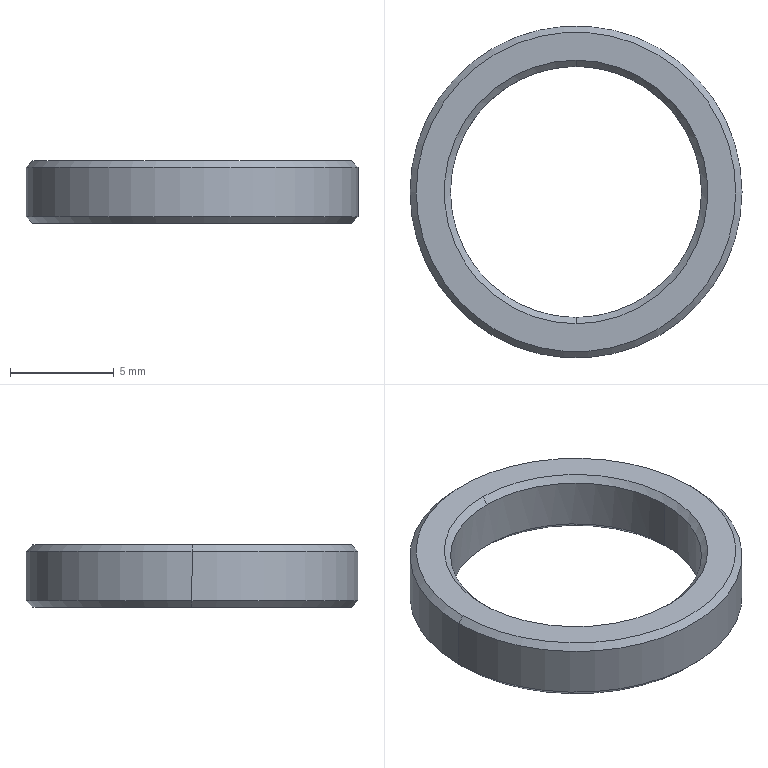Part | SolidWorks | features BaseBody 1 | 1 solid | 14 faces | box 16 x 16 x 3 mm | volume 250.27 mm3 | cone 8 | cylinder 4 | plane 2 | commonest cylinder face diameters 12.1 x2 16 x2
STEP:
#1=CARTESIAN_POINT('',(-8.,0.,2.7));
#2=VERTEX_POINT('',#1);
#3=CARTESIAN_POINT('',(8.,0.,2.7));
#4=VERTEX_POINT('',#3);
#5=CARTESIAN_POINT('',(0.,0.,2.7));
#6=DIRECTION('',(0.,0.,-1.));
#7=DIRECTION('',(-1.,0.,0.));
#8=AXIS2_PLACEMENT_3D('',#5,#6,#7);
#9=CIRCLE('',#8,8.);
#10=EDGE_CURVE('',#2,#4,#9,.T.);
#11=ORIENTED_EDGE('',*,*,#10,.T.);
#12=CARTESIAN_POINT('',(8.,0.,0.3));
#13=VERTEX_POINT('',#12);
#14=CARTESIAN_POINT('',(8.,0.,3.));
#15=DIRECTION('',(0.,0.,-1.));
#16=VECTOR('',#15,1000.);
#17=LINE('',#14,#16);
#18=EDGE_CURVE('',#4,#13,#17,.T.);
#19=ORIENTED_EDGE('',*,*,#18,.T.);
#20=CARTESIAN_POINT('',(-8.,0.,0.3));
#21=VERTEX_POINT('',#20);
#22=CARTESIAN_POINT('',(0.,0.,0.3));
#23=DIRECTION('',(0.,0.,1.));
#24=DIRECTION('',(-1.,0.,0.));
#25=AXIS2_PLACEMENT_3D('',#22,#23,#24);
#26=CIRCLE('',#25,8.);
#27=EDGE_CURVE('',#13,#21,#26,.T.);
#28=ORIENTED_EDGE('',*,*,#27,.T.);
#29=CARTESIAN_POINT('',(-8.,0.,3.));
#30=DIRECTION('',(0.,0.,-1.));
#31=VECTOR('',#30,1000.);
#32=LINE('',#29,#31);
#33=EDGE_CURVE('',#2,#21,#32,.T.);
#34=ORIENTED_EDGE('',*,*,#33,.F.);
#35=EDGE_LOOP('',(#11,#19,#28,#34));
#36=FACE_OUTER_BOUND('',#35,.T.);
#37=CARTESIAN_POINT('',(0.,0.,3.));
#38=DIRECTION('',(0.,0.,-1.));
#39=DIRECTION('',(-1.,0.,0.));
#40=AXIS2_PLACEMENT_3D('',#37,#38,#39);
#41=CYLINDRICAL_SURFACE('',#40,8.);
#42=ADVANCED_FACE('',(#36),#41,.T.);
#43=CARTESIAN_POINT('',(7.7,0.,0.));
#44=VERTEX_POINT('',#43);
#45=CARTESIAN_POINT('',(-7.7,0.,0.));
#46=VERTEX_POINT('',#45);
#47=CARTESIAN_POINT('',(0.,0.,0.));
#48=DIRECTION('',(0.,0.,1.));
#49=DIRECTION('',(1.,0.,0.));
#50=AXIS2_PLACEMENT_3D('',#47,#48,#49);
#51=CIRCLE('',#50,7.7);
#52=EDGE_CURVE('',#44,#46,#51,.T.);
#53=ORIENTED_EDGE('',*,*,#52,.T.);
#54=CARTESIAN_POINT('',(-8.,0.,0.3));
#55=DIRECTION('',(-0.7071,0.,0.7071));
#56=VECTOR('',#55,1000.);
#57=LINE('',#54,#56);
#58=EDGE_CURVE('',#46,#21,#57,.T.);
#59=ORIENTED_EDGE('',*,*,#58,.T.);
#60=ORIENTED_EDGE('',*,*,#27,.F.);
#61=CARTESIAN_POINT('',(8.,0.,0.3));
#62=DIRECTION('',(0.7071,0.,0.7071));
#63=VECTOR('',#62,1000.);
#64=LINE('',#61,#63);
#65=EDGE_CURVE('',#44,#13,#64,.T.);
#66=ORIENTED_EDGE('',*,*,#65,.F.);
#67=EDGE_LOOP('',(#53,#59,#60,#66));
#68=FACE_OUTER_BOUND('',#67,.T.);
#69=CARTESIAN_POINT('',(0.,0.,0.3));
#70=DIRECTION('',(0.,0.,1.));
#71=DIRECTION('',(1.,0.,0.));
#72=AXIS2_PLACEMENT_3D('',#69,#70,#71);
#73=CONICAL_SURFACE('',#72,8.,0.7854);
#74=ADVANCED_FACE('',(#68),#73,.T.);
#75=CARTESIAN_POINT('',(-7.7,0.,3.));
#76=VERTEX_POINT('',#75);
#77=CARTESIAN_POINT('',(7.7,0.,3.));
#78=VERTEX_POINT('',#77);
#79=CARTESIAN_POINT('',(0.,0.,3.));
#80=DIRECTION('',(0.,0.,-1.));
#81=DIRECTION('',(-1.,0.,0.));
#82=AXIS2_PLACEMENT_3D('',#79,#80,#81);
#83=CIRCLE('',#82,7.7);
#84=EDGE_CURVE('',#76,#78,#83,.T.);
#85=ORIENTED_EDGE('',*,*,#84,.T.);
#86=CARTESIAN_POINT('',(8.,0.,2.7));
#87=DIRECTION('',(0.7071,0.,-0.7071));
#88=VECTOR('',#87,1000.);
#89=LINE('',#86,#88);
#90=EDGE_CURVE('',#78,#4,#89,.T.);
#91=ORIENTED_EDGE('',*,*,#90,.T.);
#92=ORIENTED_EDGE('',*,*,#10,.F.);
#93=CARTESIAN_POINT('',(-8.,0.,2.7));
#94=DIRECTION('',(-0.7071,0.,-0.7071));
#95=VECTOR('',#94,1000.);
#96=LINE('',#93,#95);
#97=EDGE_CURVE('',#76,#2,#96,.T.);
#98=ORIENTED_EDGE('',*,*,#97,.F.);
#99=EDGE_LOOP('',(#85,#91,#92,#98));
#100=FACE_OUTER_BOUND('',#99,.T.);
#101=CARTESIAN_POINT('',(0.,0.,2.7));
#102=DIRECTION('',(0.,0.,-1.));
#103=DIRECTION('',(-1.,0.,0.));
#104=AXIS2_PLACEMENT_3D('',#101,#102,#103);
#105=CONICAL_SURFACE('',#104,8.,0.7854);
#106=ADVANCED_FACE('',(#100),#105,.T.);
#107=CARTESIAN_POINT('',(6.05,0.,0.3));
#108=VERTEX_POINT('',#107);
#109=CARTESIAN_POINT('',(-6.05,0.,0.3));
#110=VERTEX_POINT('',#109);
#111=CARTESIAN_POINT('',(0.,0.,0.3));
#112=DIRECTION('',(0.,0.,-1.));
#113=DIRECTION('',(-1.,0.,0.));
#114=AXIS2_PLACEMENT_3D('',#111,#112,#113);
#115=CIRCLE('',#114,6.05);
#116=EDGE_CURVE('',#108,#110,#115,.T.);
#117=ORIENTED_EDGE('',*,*,#116,.F.);
#118=CARTESIAN_POINT('',(6.35,0.,0.));
#119=VERTEX_POINT('',#118);
#120=CARTESIAN_POINT('',(6.35,0.,0.));
#121=DIRECTION('',(0.7071,0.,-0.7071));
#122=VECTOR('',#121,1000.);
#123=LINE('',#120,#122);
#124=EDGE_CURVE('',#108,#119,#123,.T.);
#125=ORIENTED_EDGE('',*,*,#124,.T.);
#126=CARTESIAN_POINT('',(-6.35,0.,0.));
#127=VERTEX_POINT('',#126);
#128=CARTESIAN_POINT('',(0.,0.,0.));
#129=DIRECTION('',(0.,0.,-1.));
#130=DIRECTION('',(-1.,0.,0.));
#131=AXIS2_PLACEMENT_3D('',#128,#129,#130);
#132=CIRCLE('',#131,6.35);
#133=EDGE_CURVE('',#119,#127,#132,.T.);
#134=ORIENTED_EDGE('',*,*,#133,.T.);
#135=CARTESIAN_POINT('',(-6.35,0.,0.));
#136=DIRECTION('',(-0.7071,0.,-0.7071));
#137=VECTOR('',#136,1000.);
#138=LINE('',#135,#137);
#139=EDGE_CURVE('',#110,#127,#138,.T.);
#140=ORIENTED_EDGE('',*,*,#139,.F.);
#141=EDGE_LOOP('',(#117,#125,#134,#140));
#142=FACE_OUTER_BOUND('',#141,.T.);
#143=CARTESIAN_POINT('',(0.,0.,0.));
#144=DIRECTION('',(0.,0.,-1.));
#145=DIRECTION('',(-1.,0.,0.));
#146=AXIS2_PLACEMENT_3D('',#143,#144,#145);
#147=CONICAL_SURFACE('',#146,6.35,0.7854);
#148=ADVANCED_FACE('',(#142),#147,.F.);
#149=CARTESIAN_POINT('',(0.,6.05,2.7));
#150=VERTEX_POINT('',#149);
#151=CARTESIAN_POINT('',(-6.05,0.,2.7));
#152=VERTEX_POINT('',#151);
#153=CARTESIAN_POINT('',(0.,0.,2.7));
#154=DIRECTION('',(0.,0.,1.));
#155=DIRECTION('',(1.,0.,0.));
#156=AXIS2_PLACEMENT_3D('',#153,#154,#155);
#157=CIRCLE('',#156,6.05);
#158=EDGE_CURVE('',#150,#152,#157,.T.);
#159=ORIENTED_EDGE('',*,*,#158,.F.);
#160=CARTESIAN_POINT('',(0.,6.35,3.));
#161=VERTEX_POINT('',#160);
#162=CARTESIAN_POINT('',(0.,6.35,3.));
#163=DIRECTION('',(0.,0.7071,0.7071));
#164=VECTOR('',#163,1000.);
#165=LINE('',#162,#164);
#166=EDGE_CURVE('',#150,#161,#165,.T.);
#167=ORIENTED_EDGE('',*,*,#166,.T.);
#168=CARTESIAN_POINT('',(0.,-6.35,3.));
#169=VERTEX_POINT('',#168);
#170=CARTESIAN_POINT('',(0.,0.,3.));
#171=DIRECTION('',(0.,0.,-1.));
#172=DIRECTION('',(0.,-1.,0.));
#173=AXIS2_PLACEMENT_3D('',#170,#171,#172);
#174=CIRCLE('',#173,6.35);
#175=EDGE_CURVE('',#169,#161,#174,.T.);
#176=ORIENTED_EDGE('',*,*,#175,.F.);
#177=CARTESIAN_POINT('',(0.,-6.05,2.7));
#178=VERTEX_POINT('',#177);
#179=CARTESIAN_POINT('',(0.,-6.35,3.));
#180=DIRECTION('',(0.,-0.7071,0.7071));
#181=VECTOR('',#180,1000.);
#182=LINE('',#179,#181);
#183=EDGE_CURVE('',#178,#169,#182,.T.);
#184=ORIENTED_EDGE('',*,*,#183,.F.);
#185=CARTESIAN_POINT('',(0.,0.,2.7));
#186=DIRECTION('',(0.,0.,1.));
#187=DIRECTION('',(1.,0.,0.));
#188=AXIS2_PLACEMENT_3D('',#185,#186,#187);
#189=CIRCLE('',#188,6.05);
#190=EDGE_CURVE('',#152,#178,#189,.T.);
#191=ORIENTED_EDGE('',*,*,#190,.F.);
#192=EDGE_LOOP('',(#159,#167,#176,#184,#191));
#193=FACE_OUTER_BOUND('',#192,.T.);
#194=CARTESIAN_POINT('',(0.,0.,3.));
#195=DIRECTION('',(0.,0.,1.));
#196=DIRECTION('',(0.,-1.,0.));
#197=AXIS2_PLACEMENT_3D('',#194,#195,#196);
#198=CONICAL_SURFACE('',#197,6.35,0.7854);
#199=ADVANCED_FACE('',(#193),#198,.F.);
#200=ORIENTED_EDGE('',*,*,#190,.T.);
#201=CARTESIAN_POINT('',(6.05,0.,2.7));
#202=VERTEX_POINT('',#201);
#203=CARTESIAN_POINT('',(0.,0.,2.7));
#204=DIRECTION('',(0.,0.,1.));
#205=DIRECTION('',(1.,0.,0.));
#206=AXIS2_PLACEMENT_3D('',#203,#204,#205);
#207=CIRCLE('',#206,6.05);
#208=EDGE_CURVE('',#178,#202,#207,.T.);
#209=ORIENTED_EDGE('',*,*,#208,.T.);
#210=CARTESIAN_POINT('',(6.05,0.,3.));
#211=DIRECTION('',(0.,0.,-1.));
#212=VECTOR('',#211,1000.);
#213=LINE('',#210,#212);
#214=EDGE_CURVE('',#202,#108,#213,.T.);
#215=ORIENTED_EDGE('',*,*,#214,.T.);
#216=ORIENTED_EDGE('',*,*,#116,.T.);
#217=CARTESIAN_POINT('',(-6.05,0.,3.));
#218=DIRECTION('',(0.,0.,-1.));
#219=VECTOR('',#218,1000.);
#220=LINE('',#217,#219);
#221=EDGE_CURVE('',#152,#110,#220,.T.);
#222=ORIENTED_EDGE('',*,*,#221,.F.);
#223=EDGE_LOOP('',(#200,#209,#215,#216,#222));
#224=FACE_OUTER_BOUND('',#223,.T.);
#225=CARTESIAN_POINT('',(0.,0.,3.));
#226=DIRECTION('',(0.,0.,-1.));
#227=DIRECTION('',(-1.,0.,0.));
#228=AXIS2_PLACEMENT_3D('',#225,#226,#227);
#229=CYLINDRICAL_SURFACE('',#228,6.05);
#230=ADVANCED_FACE('',(#224),#229,.F.);
#231=ORIENTED_EDGE('',*,*,#18,.F.);
#232=CARTESIAN_POINT('',(0.,0.,2.7));
#233=DIRECTION('',(0.,0.,-1.));
#234=DIRECTION('',(-1.,0.,0.));
#235=AXIS2_PLACEMENT_3D('',#232,#233,#234);
#236=CIRCLE('',#235,8.);
#237=EDGE_CURVE('',#4,#2,#236,.T.);
#238=ORIENTED_EDGE('',*,*,#237,.T.);
#239=ORIENTED_EDGE('',*,*,#33,.T.);
#240=CARTESIAN_POINT('',(0.,0.,0.3));
#241=DIRECTION('',(0.,0.,1.));
#242=DIRECTION('',(-1.,0.,0.));
#243=AXIS2_PLACEMENT_3D('',#240,#241,#242);
#244=CIRCLE('',#243,8.);
#245=EDGE_CURVE('',#21,#13,#244,.T.);
#246=ORIENTED_EDGE('',*,*,#245,.T.);
#247=EDGE_LOOP('',(#231,#238,#239,#246));
#248=FACE_OUTER_BOUND('',#247,.T.);
#249=CARTESIAN_POINT('',(0.,0.,3.));
#250=DIRECTION('',(0.,0.,-1.));
#251=DIRECTION('',(-1.,0.,0.));
#252=AXIS2_PLACEMENT_3D('',#249,#250,#251);
#253=CYLINDRICAL_SURFACE('',#252,8.);
#254=ADVANCED_FACE('',(#248),#253,.T.);
#255=ORIENTED_EDGE('',*,*,#58,.F.);
#256=CARTESIAN_POINT('',(0.,0.,0.));
#257=DIRECTION('',(0.,0.,1.));
#258=DIRECTION('',(1.,0.,0.));
#259=AXIS2_PLACEMENT_3D('',#256,#257,#258);
#260=CIRCLE('',#259,7.7);
#261=EDGE_CURVE('',#46,#44,#260,.T.);
#262=ORIENTED_EDGE('',*,*,#261,.T.);
#263=ORIENTED_EDGE('',*,*,#65,.T.);
#264=ORIENTED_EDGE('',*,*,#245,.F.);
#265=EDGE_LOOP('',(#255,#262,#263,#264));
#266=FACE_OUTER_BOUND('',#265,.T.);
#267=CARTESIAN_POINT('',(0.,0.,0.3));
#268=DIRECTION('',(0.,0.,1.));
#269=DIRECTION('',(1.,0.,0.));
#270=AXIS2_PLACEMENT_3D('',#267,#268,#269);
#271=CONICAL_SURFACE('',#270,8.,0.7854);
#272=ADVANCED_FACE('',(#266),#271,.T.);
#273=ORIENTED_EDGE('',*,*,#90,.F.);
#274=CARTESIAN_POINT('',(0.,0.,3.));
#275=DIRECTION('',(0.,0.,-1.));
#276=DIRECTION('',(-1.,0.,0.));
#277=AXIS2_PLACEMENT_3D('',#274,#275,#276);
#278=CIRCLE('',#277,7.7);
#279=EDGE_CURVE('',#78,#76,#278,.T.);
#280=ORIENTED_EDGE('',*,*,#279,.T.);
#281=ORIENTED_EDGE('',*,*,#97,.T.);
#282=ORIENTED_EDGE('',*,*,#237,.F.);
#283=EDGE_LOOP('',(#273,#280,#281,#282));
#284=FACE_OUTER_BOUND('',#283,.T.);
#285=CARTESIAN_POINT('',(0.,0.,2.7));
#286=DIRECTION('',(0.,0.,-1.));
#287=DIRECTION('',(-1.,0.,0.));
#288=AXIS2_PLACEMENT_3D('',#285,#286,#287);
#289=CONICAL_SURFACE('',#288,8.,0.7854);
#290=ADVANCED_FACE('',(#284),#289,.T.);
#291=CARTESIAN_POINT('',(0.,0.,0.));
#292=DIRECTION('',(0.,0.,-1.));
#293=DIRECTION('',(-1.,0.,0.));
#294=AXIS2_PLACEMENT_3D('',#291,#292,#293);
#295=CIRCLE('',#294,6.35);
#296=EDGE_CURVE('',#127,#119,#295,.T.);
#297=ORIENTED_EDGE('',*,*,#296,.F.);
#298=ORIENTED_EDGE('',*,*,#133,.F.);
#299=EDGE_LOOP('',(#297,#298));
#300=FACE_BOUND('',#299,.T.);
#301=ORIENTED_EDGE('',*,*,#52,.F.);
#302=ORIENTED_EDGE('',*,*,#261,.F.);
#303=EDGE_LOOP('',(#301,#302));
#304=FACE_OUTER_BOUND('',#303,.T.);
#305=CARTESIAN_POINT('',(0.,0.,0.));
#306=DIRECTION('',(0.,0.,1.));
#307=DIRECTION('',(1.,0.,0.));
#308=AXIS2_PLACEMENT_3D('',#305,#306,#307);
#309=PLANE('',#308);
#310=ADVANCED_FACE('',(#300,#304),#309,.F.);
#311=ORIENTED_EDGE('',*,*,#84,.F.);
#312=ORIENTED_EDGE('',*,*,#279,.F.);
#313=EDGE_LOOP('',(#311,#312));
#314=FACE_OUTER_BOUND('',#313,.T.);
#315=ORIENTED_EDGE('',*,*,#175,.T.);
#316=CARTESIAN_POINT('',(0.,0.,3.));
#317=DIRECTION('',(0.,0.,-1.));
#318=DIRECTION('',(0.,-1.,0.));
#319=AXIS2_PLACEMENT_3D('',#316,#317,#318);
#320=CIRCLE('',#319,6.35);
#321=EDGE_CURVE('',#161,#169,#320,.T.);
#322=ORIENTED_EDGE('',*,*,#321,.T.);
#323=EDGE_LOOP('',(#315,#322));
#324=FACE_BOUND('',#323,.T.);
#325=CARTESIAN_POINT('',(0.,0.,3.));
#326=DIRECTION('',(0.,0.,1.));
#327=DIRECTION('',(1.,0.,0.));
#328=AXIS2_PLACEMENT_3D('',#325,#326,#327);
#329=PLANE('',#328);
#330=ADVANCED_FACE('',(#314,#324),#329,.T.);
#331=ORIENTED_EDGE('',*,*,#124,.F.);
#332=CARTESIAN_POINT('',(0.,0.,0.3));
#333=DIRECTION('',(0.,0.,-1.));
#334=DIRECTION('',(-1.,0.,0.));
#335=AXIS2_PLACEMENT_3D('',#332,#333,#334);
#336=CIRCLE('',#335,6.05);
#337=EDGE_CURVE('',#110,#108,#336,.T.);
#338=ORIENTED_EDGE('',*,*,#337,.F.);
#339=ORIENTED_EDGE('',*,*,#139,.T.);
#340=ORIENTED_EDGE('',*,*,#296,.T.);
#341=EDGE_LOOP('',(#331,#338,#339,#340));
#342=FACE_OUTER_BOUND('',#341,.T.);
#343=CARTESIAN_POINT('',(0.,0.,0.));
#344=DIRECTION('',(0.,0.,-1.));
#345=DIRECTION('',(-1.,0.,0.));
#346=AXIS2_PLACEMENT_3D('',#343,#344,#345);
#347=CONICAL_SURFACE('',#346,6.35,0.7854);
#348=ADVANCED_FACE('',(#342),#347,.F.);
#349=ORIENTED_EDGE('',*,*,#166,.F.);
#350=CARTESIAN_POINT('',(0.,0.,2.7));
#351=DIRECTION('',(0.,0.,1.));
#352=DIRECTION('',(1.,0.,0.));
#353=AXIS2_PLACEMENT_3D('',#350,#351,#352);
#354=CIRCLE('',#353,6.05);
#355=EDGE_CURVE('',#202,#150,#354,.T.);
#356=ORIENTED_EDGE('',*,*,#355,.F.);
#357=ORIENTED_EDGE('',*,*,#208,.F.);
#358=ORIENTED_EDGE('',*,*,#183,.T.);
#359=ORIENTED_EDGE('',*,*,#321,.F.);
#360=EDGE_LOOP('',(#349,#356,#357,#358,#359));
#361=FACE_OUTER_BOUND('',#360,.T.);
#362=CARTESIAN_POINT('',(0.,0.,3.));
#363=DIRECTION('',(0.,0.,1.));
#364=DIRECTION('',(0.,-1.,0.));
#365=AXIS2_PLACEMENT_3D('',#362,#363,#364);
#366=CONICAL_SURFACE('',#365,6.35,0.7854);
#367=ADVANCED_FACE('',(#361),#366,.F.);
#368=ORIENTED_EDGE('',*,*,#214,.F.);
#369=ORIENTED_EDGE('',*,*,#355,.T.);
#370=ORIENTED_EDGE('',*,*,#158,.T.);
#371=ORIENTED_EDGE('',*,*,#221,.T.);
#372=ORIENTED_EDGE('',*,*,#337,.T.);
#373=EDGE_LOOP('',(#368,#369,#370,#371,#372));
#374=FACE_OUTER_BOUND('',#373,.T.);
#375=CARTESIAN_POINT('',(0.,0.,3.));
#376=DIRECTION('',(0.,0.,-1.));
#377=DIRECTION('',(-1.,0.,0.));
#378=AXIS2_PLACEMENT_3D('',#375,#376,#377);
#379=CYLINDRICAL_SURFACE('',#378,6.05);
#380=ADVANCED_FACE('',(#374),#379,.F.);
#381=CLOSED_SHELL('',(#42,#74,#106,#148,#199,#230,#254,#272,#290,#310,#330,#348,#367,#380));
#382=MANIFOLD_SOLID_BREP('',#381);
#383=CARTESIAN_POINT('',(0.,0.,0.));
#384=DIRECTION('',(0.,0.,1.));
#385=DIRECTION('',(1.,0.,0.));
#386=AXIS2_PLACEMENT_3D('',#383,#384,#385);
#387=(LENGTH_UNIT()NAMED_UNIT(*)SI_UNIT(.MILLI.,.METRE.));
#388=UNCERTAINTY_MEASURE_WITH_UNIT(LENGTH_MEASURE(0.00001),#387,'','');
#389=(NAMED_UNIT(*)PLANE_ANGLE_UNIT()SI_UNIT($,.RADIAN.));
#390=(NAMED_UNIT(*)SI_UNIT($,.STERADIAN.)SOLID_ANGLE_UNIT());
#391=(GEOMETRIC_REPRESENTATION_CONTEXT(3)GLOBAL_UNCERTAINTY_ASSIGNED_CONTEXT((#388))GLOBAL_UNIT_ASSIGNED_CONTEXT((#387,#389,#390))REPRESENTATION_CONTEXT('',''));
#392=ADVANCED_BREP_SHAPE_REPRESENTATION('',(#382,#386),#391);